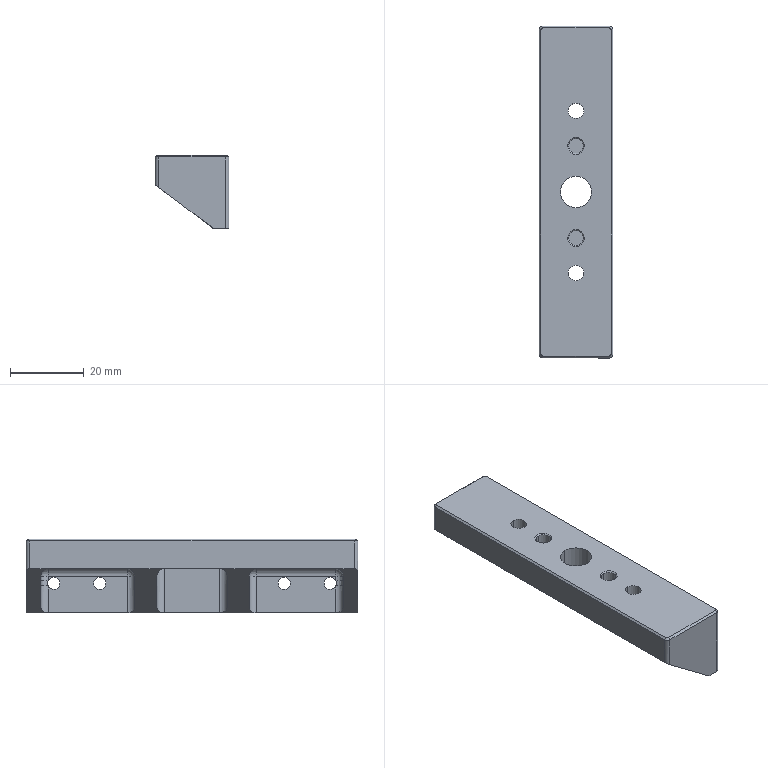NC program | NX | posted with a generic post | part box 20 x 90 x 20 mm
Lines 1 to 774 of 15930:
N10 G17 G21 G94 G90
(FLOOR_WALL_COPY , TOOL : D80)
N12 T19 M6
N14 G54
N16 G17 G0 G90 X-88. Y0. B0. C0. S6500 M3
N18 G43 Z30. H19
N20 Z7.
N22 G94 G1 Z4. F1500.
N24 X-85.
N26 X85.
N28 X88.
N30 Z7.
N32 G0 Z30.
N34 X-88.
N36 Z6.
N38 G1 Z3.
N40 X-85.
N42 X85.
N44 X88.
N46 Z6.
N48 G0 Z30.
N50 X-88.
N52 Z5.
N54 G1 Z2.
N56 X-85.
N58 X85.
N60 X88.
N62 Z5.
N64 G0 Z30.
N66 X-88.
N68 Z4.
N70 G1 Z1.
N72 X-85.
N74 X85.
N76 X88.
N78 Z4.
N80 G0 Z30.
N82 X-88.
N84 Z3.
N86 G1 Z0.
N88 X-85.
N90 X85.
N92 X88.
N94 Z3.
N96 G0 Z30.
N98 M5
(CAVITY_MILL , TOOL : D10)
N100 T15 M6
N102 G54
N104 G17 G0 G90 X4.33 Y-16.996 B0. C0. S9500 M3
N106 G43 Z30. H15
N108 Z0.508
N110 G94 G1 Z-0.992 F1000.
N112 X0.866 Y-10.996
N114 G3 X0. Y-10.496 R1.
N116 G1 Y-5.996
N118 X40.997 F3500.
N120 Y-4.989
N122 G2 X35.946 Y-3.6 R9.462
N124 G1 X20.574
N126 G2 X15.58 Y-4.989 R9.612
N128 G1 X9.359
N130 G2 X4.437 Y-3.6 R10.03
N132 G1 X-4.432
N134 G2 X-9.412 Y-4.989 R9.663
N136 G1 X-15.662
N138 G2 X-20.59 Y-3.6 R10.353
N140 G1 X-35.931
N142 G2 X-40.895 Y-4.989 R9.801
N144 G1 X-40.997
N146 Y-5.996
N148 X0.
N150 Y-10.496
N152 X45.004
N154 G3 X45.497 Y-10.003 R0.493
N156 G1 Y-1.867
N158 G3 X49.997 Y0.476 R6.533
N160 G1 Y3.622
N162 G2 X45. Y-0.489 R5.133
N164 G1 X40.881
N166 G2 X38.089 Y0.371 R4.962
N168 X37.347 Y0.9 R21.375
N170 G1 X19.1
N172 G2 X15.585 Y-0.489 R5.112
N174 G1 X9.409
N176 G2 X5.865 Y0.9 R5.53
N178 G1 X-5.9
N180 G2 X-9.415 Y-0.489 R5.163
N182 G1 X-15.591
N184 G2 X-19.194 Y0.9 R5.853
N186 G1 X-37.384
N188 G2 X-40.997 Y-0.489 R5.301
N190 G1 X-45.
N192 G2 X-49.997 Y3.622 R5.133
N194 G1 Y0.476
N196 G3 X-45.497 Y-1.867 R6.533
N198 G1 Y-10.003
N200 G3 X-45.004 Y-10.496 R0.493
N202 G1 X0.
N204 G2 X0.866 Y-10.996 R1.
N206 G1 X4.33 Y-16.996
N208 Z0.508
N210 G0 X32.575 Z-0.483
N212 G1 Z-1.983 F1000.
N214 X29.111 Y-10.996
N216 G3 X28.245 Y-10.496 R1.
N218 G1 Y-5.996
N220 X38.636 F3500.
N222 G2 X34.338 Y-3.6 R9.795
N224 G1 X22.164
N226 G2 X17.854 Y-5.996 R9.845
N228 G1 X28.245
N230 Y-10.496
N232 X45.004
N234 G3 X45.497 Y-10.003 R0.494
N236 G1 Y-3.187
N238 G3 X49.997 Y-0.827 R6.564
N240 G1 Y2.328
N242 G2 X45. Y-1.811 R5.164
N244 G1 X41.
N246 G2 X36.481 Y0.9 R5.295
N248 G1 X20.03
N250 G2 X15.5 Y-1.811 R5.345
N252 G1 X9.5
N254 G2 X8.216 Y-1.644 R5.087
N256 G1 X7.072 Y-5.996
N258 G2 X2.828 Y-3.6 R9.587
N260 G1 X-2.829
N262 G2 X-7.069 Y-5.996 R9.575
N264 G1 X7.072
N266 X8.216 Y-1.644
N268 G2 X5.011 Y0.9 R5.087
N270 G1 X-5.014
N272 G2 X-9.5 Y-1.811 R5.075
N274 G1 X-15.5
N276 G2 X-16.78 Y-1.644 R5.113
N278 G1 X-17.923 Y-5.996
N280 G2 X-22.174 Y-3.6 R9.613
N282 G1 X-34.338
N284 G2 X-38.636 Y-5.996 R9.795
N286 G1 X-17.923
N288 X-16.78 Y-1.644
N290 G2 X-19.996 Y0.9 R5.113
N292 G1 X-36.481
N294 G2 X-41. Y-1.811 R5.295
N296 G1 X-45.033
N298 G2 X-49.997 Y2.331 R5.167
N300 G1 Y-0.825
N302 G3 X-45.497 Y-3.187 R6.567
N304 G1 Y-10.003
N306 G3 X-45.004 Y-10.496 R0.494
N308 G1 X28.245
N310 G2 X29.111 Y-10.996 R1.
N312 G1 X32.575 Y-16.996
N314 Z-0.483
N316 G0 X32.581 Z-1.475
N318 G1 Z-2.975 F1000.
N320 X29.117 Y-10.996
N322 G3 X28.251 Y-10.496 R1.
N324 G1 Y-5.996
N326 X35.657 F3500.
N328 G2 X33.194 Y-3.6 R9.616
N330 G1 X23.307
N332 G2 X20.845 Y-5.996 R9.612
N334 G1 X28.251
N336 Y-10.496
N338 X45.004
N340 G3 X45.497 Y-10.002 R0.494
N342 G1 Y-4.512
N344 G3 X49.997 Y-2.169 R6.533
N346 G1 Y0.979
N348 G2 X45. Y-3.133 R5.133
N350 G1 X41.
N352 G2 X36.023 Y0.9 R5.116
N354 G1 X20.476
N356 G2 X15.5 Y-3.133 R5.112
N358 G1 X9.5
N360 G2 X6.666 Y-2.263 R5.105
N362 G1 X4.153 Y-5.996
N364 G2 X1.693 Y-3.6 R9.605
N366 G1 X-1.693
N368 G2 X-4.153 Y-5.996 R9.605
N370 G1 X4.153
N372 X6.666 Y-2.263
N374 G2 X4.525 Y0.9 R5.105
N376 G1 X-4.525
N378 G2 X-9.5 Y-3.133 R5.105
N380 G1 X-15.5
N382 G2 X-18.333 Y-2.263 R5.113
N384 G1 X-20.845 Y-5.996
N386 G2 X-23.307 Y-3.6 R9.613
N388 G1 X-33.194
N390 G2 X-35.656 Y-5.996 R9.615
N392 G1 X-20.845
N394 X-18.333 Y-2.263
N396 G2 X-20.477 Y0.9 R5.113
N398 G1 X-36.024
N400 G2 X-41. Y-3.133 R5.115
N402 G1 X-45.019
N404 G2 X-49.997 Y0.981 R5.136
N406 G1 Y-2.167
N408 G3 X-45.497 Y-4.512 R6.536
N410 G1 Y-10.002
N412 G3 X-45.004 Y-10.496 R0.494
N414 G1 X28.251
N416 G2 X29.117 Y-10.996 R1.
N418 G1 X32.581 Y-16.996
N420 Z-1.475
N422 G0 X32.58 Y-16.997 Z-2.467
N424 G1 Z-3.967 F1000.
N426 X29.116 Y-10.997
N428 G3 X28.25 Y-10.497 R1.
N430 G1 Y-5.997
N432 X34.087 F3500.
N434 G2 X32.402 Y-3.6 R9.633
N436 G1 X24.098
N438 G2 X22.413 Y-5.997 R9.633
N440 G1 X28.25
N442 Y-10.497
N444 X45.003
N446 G3 X45.498 Y-10.002 R0.494
N448 G1 Y-5.834
N450 G3 X49.998 Y-3.491 R6.533
N452 G1 Y-0.343
N454 G2 X45. Y-4.456 R5.133
N456 G1 X41.
N458 G2 X35.9 Y0.711 R5.133
N460 G1 Y0.9
N462 X20.6
N464 Y0.711
N466 G2 X15.5 Y-4.456 R5.133
N468 G1 X9.5
N470 G2 X5.832 Y-2.879 R5.133
N472 G1 X2.587 Y-5.997
N474 G2 X0.902 Y-3.6 R9.633
N476 G1 X-0.902
N478 G2 X-2.587 Y-5.997 R9.633
N480 G1 X2.587
N482 X5.832 Y-2.879
N484 G2 X4.517 Y-0.413 R5.133
N486 X4.4 Y0.756 R5.134
N488 G1 X4.401 Y0.9
N490 X-4.4
N492 Y0.711
N494 G2 X-9.5 Y-4.456 R5.133
N496 G1 X-15.5
N498 G2 X-19.168 Y-2.879 R5.133
N500 G1 X-22.413 Y-5.997
N502 G2 X-24.098 Y-3.6 R9.633
N504 G1 X-32.402
N506 G2 X-34.087 Y-5.997 R9.633
N508 G1 X-22.413
N510 X-19.168 Y-2.879
N512 G2 X-20.6 Y0.711 R5.133
N514 G1 Y0.9
N516 X-35.9
N518 Y0.711
N520 G2 X-41. Y-4.456 R5.133
N522 G1 X-45.
N524 G2 X-49.998 Y-0.343 R5.133
N526 G1 Y-3.491
N528 G3 X-45.498 Y-5.834 R6.533
N530 G1 Y-10.002
N532 G3 X-45.003 Y-10.497 R0.494
N534 G1 X28.25
N536 G2 X29.116 Y-10.997 R1.
N538 G1 X32.58 Y-16.997
N540 Z-2.467
N542 G0 X32.581 Z-3.458
N544 G1 Z-4.958 F1000.
N546 X29.117 Y-10.997
N548 G3 X28.251 Y-10.497 R1.
N550 G1 Y-5.997
N552 X33.027 F3500.
N554 G2 X31.867 Y-3.6 R9.641
N556 G1 X24.635
N558 G2 X23.475 Y-5.997 R9.636
N560 G1 X28.251
N562 Y-10.497
N564 X45.003
N566 G3 X45.498 Y-10.002 R0.494
N568 G1 Y-7.154
N570 G3 X49.998 Y-4.793 R6.565
N572 G1 Y-1.636
N574 G2 X45. Y-5.778 R5.165
N576 G1 X41.
N578 G2 X35.9 Y-0.611 R5.141
N580 G1 Y0.9
N582 X20.6
N584 Y-0.611
N586 G2 X15.5 Y-5.778 R5.136
N588 G1 X9.5
N590 G2 X5.279 Y-3.488 R5.175
N592 G1 X1.543 Y-5.997
N594 G2 X0.376 Y-3.6 R9.675
N596 G1 X-0.376
N598 G2 X-1.543 Y-5.997 R9.675
N600 G1 X1.543
N602 X5.279 Y-3.488
N604 G2 X4.4 Y-0.611 R5.175
N606 G1 Y0.9
N608 X-4.4
N610 Y-0.611
N612 G2 X-9.5 Y-5.778 R5.175
N614 G1 X-15.5
N616 G2 X-19.734 Y-3.496 R5.136
N618 G1 X-23.475 Y-5.997
N620 G2 X-24.635 Y-3.6 R9.636
N622 G1 X-31.867
N624 G2 X-33.027 Y-5.997 R9.641
N626 G1 X-23.475
N628 X-19.734 Y-3.496
N630 G2 X-20.6 Y-0.611 R5.136
N632 G1 Y0.9
N634 X-35.9
N636 Y-0.611
N638 G2 X-41. Y-5.778 R5.141
N640 G1 X-45.
N642 G2 X-49.998 Y-1.634 R5.167
N644 G1 Y-4.791
N646 G3 X-45.498 Y-7.154 R6.567
N648 G1 Y-10.002
N650 G3 X-45.003 Y-10.497 R0.494
N652 G1 X28.251
N654 G2 X29.117 Y-10.997 R1.
N656 G1 X32.581 Y-16.997
N658 Z-3.458
N660 G0 X32.582 Z-4.45
N662 G1 Z-5.95 F1000.
N664 X29.118 Y-10.997
N666 G3 X28.252 Y-10.497 R1.
N668 G1 Y-5.997
N670 X32.287 F3500.
N672 G2 X31.541 Y-3.6 R9.644
N674 G1 X24.961
N676 G2 X24.217 Y-5.997 R9.633
N678 G1 X28.252
N680 Y-10.497
N682 X45.003
N684 G3 X45.498 Y-10.002 R0.495
N686 G1 Y-8.478
N688 G3 X49.998 Y-6.129 R6.543
N690 G1 Y-2.977
N692 G2 X45. Y-7.1 R5.143
N694 G1 X41.
N696 G2 X35.9 Y-1.933 R5.144
N698 G1 Y0.9
N700 X20.6
N702 Y-1.933
N704 G2 X15.5 Y-7.1 R5.133
N706 G1 X9.5
N708 G2 X4.879 Y-4.105 R5.17
N710 G1 X0.797 Y-5.997
N712 G2 X0.045 Y-3.6 R9.67
N714 G1 X-0.045
N716 G2 X-0.797 Y-5.997 R9.67
N718 G1 X0.797
N720 X4.879 Y-4.105
N722 G2 X4.4 Y-1.933 R5.17
N724 G1 Y0.9
N726 X-4.4
N728 Y-1.933
N730 G2 X-9.5 Y-7.1 R5.17
N732 G1 X-15.533
N734 G2 X-20.129 Y-4.114 R5.133
N736 G1 X-24.217 Y-5.997
N738 G2 X-24.961 Y-3.6 R9.633
N740 G1 X-31.541
N742 G2 X-32.287 Y-5.997 R9.644
N744 G1 X-24.217
N746 X-20.129 Y-4.114
N748 G2 X-20.6 Y-1.933 R5.133
N750 G1 Y0.9
N752 X-35.9
N754 Y-1.933
N756 G2 X-41. Y-7.1 R5.144
N758 G1 X-45.
N760 G2 X-49.998 Y-2.975 R5.146
N762 G1 Y-6.127
N764 G3 X-45.498 Y-8.478 R6.546
N766 G1 Y-10.002
N768 G3 X-45.003 Y-10.497 R0.495
N770 G1 X28.252
N772 G2 X29.118 Y-10.997 R1.
N774 G1 X32.582 Y-16.997
N776 Z-4.45
N778 G0 X32.58 Z-5.442
N780 G1 Z-6.942 F1000.
N782 X29.116 Y-10.997
N784 G3 X28.25 Y-10.497 R1.
N786 G1 Y-5.997
N788 X31.788 F3500.
N790 G2 X31.405 Y-3.6 R9.633
N792 G1 X25.095
N794 G2 X24.712 Y-5.997 R9.633
N796 G1 X28.25
N798 Y-10.497
N800 X45.003
N802 G3 X45.498 Y-10.002 R0.495
N804 G1 Y-9.801
N806 G3 X49.998 Y-7.457 R6.533
N808 G1 Y-4.307
N810 G2 X45. Y-8.422 R5.133
N812 G1 X41.
N814 G2 X35.9 Y-3.256 R5.133
N816 G1 Y0.9
N818 X20.6
N820 Y-3.256
N822 G2 X15.5 Y-8.422 R5.133
N824 G1 X9.5
N826 G2 X4.607 Y-4.732 R5.133
N828 G1 X0.288 Y-5.997
N830 G2 X0. Y-4.674 R9.633
N832 X-0.288 Y-5.997 R9.633
N834 G1 X0.288
N836 X4.607 Y-4.732
N838 G2 X4.4 Y-3.256 R5.133
N840 G1 Y0.9
N842 X-4.4
N844 Y-3.256
N846 G2 X-9.5 Y-8.422 R5.133
N848 G1 X-15.5
N850 G2 X-20.393 Y-4.732 R5.133
N852 G1 X-24.712 Y-5.997
N854 G2 X-25.095 Y-3.6 R9.633
N856 G1 X-31.405
N858 G2 X-31.788 Y-5.997 R9.633
N860 G1 X-24.712
N862 X-20.393 Y-4.732
N864 G2 X-20.6 Y-3.256 R5.133
N866 G1 Y0.9
N868 X-35.9
N870 Y-3.256
N872 G2 X-41. Y-8.422 R5.133
N874 G1 X-45.
N876 G2 X-49.998 Y-4.307 R5.133
N878 G1 Y-7.457
N880 G3 X-45.498 Y-9.801 R6.533
N882 G1 Y-10.002
N884 G3 X-45.003 Y-10.497 R0.495
N886 G1 X28.25
N888 G2 X29.116 Y-10.997 R1.
N890 G1 X32.58 Y-16.997
N892 Z-5.442
N894 G0 Z-6.433
N896 G1 Z-7.933 F1000.
N898 X29.116 Y-10.997
N900 G3 X28.25 Y-10.497 R1.
N902 G1 Y-5.997
N904 X31.5 F3500.
N906 G2 X31.4 Y-4.674 R9.633
N908 G1 Y-3.6
N910 X25.1
N912 Y-4.565
N914 G2 X25. Y-5.997 R9.633
N916 G1 X28.25
N918 Y-10.497
N920 X38.198
N922 G3 X41. Y-11.144 R6.533
N924 G1 X45.012
N926 G3 X49.998 Y-8.772 R6.544
N928 G1 Y-5.619
N930 G2 X45. Y-9.744 R5.144
N932 G1 X41.
N934 G2 X35.9 Y-4.578 R5.133
N936 G1 Y0.9
N938 X20.6
N940 Y-4.644
N942 G2 X15.5 Y-9.744 R5.133
N944 G1 X9.5
N946 G2 X4.454 Y-5.346 R5.143
N948 G1 X0.001 Y-5.997
N950 X4.454 Y-5.346
N952 X4.453 Y-5.341
N954 G2 X4.4 Y-4.578 R5.143
N956 G1 Y0.9
N958 X-4.4
N960 Y-4.578
N962 G2 X-9.5 Y-9.744 R5.143
N964 G1 X-15.5
N966 G2 X-20.547 Y-5.35 R5.133
N968 G1 X-25. Y-5.997
N970 G2 X-25.1 Y-4.674 R9.633
N972 G1 Y-3.6
N974 X-31.4
N976 Y-4.565
N978 G2 X-31.5 Y-5.997 R9.633
N980 G1 X-25.
N982 X-20.547 Y-5.35
N984 G2 X-20.6 Y-4.578 R5.133
N986 G1 Y0.9
N988 X-35.9
N990 Y-4.644
N992 G2 X-41. Y-9.744 R5.133
N994 G1 X-45.
N996 G2 X-49.998 Y-5.617 R5.146
N998 G1 Y-8.771
N1000 G3 X-45. Y-11.144 R6.546
N1002 G1 X-40.991
N1004 G3 X-38.198 Y-10.497 R6.533
N1006 G1 X-18.302
N1008 G3 X-15.5 Y-11.144 R6.533
N1010 G1 X-9.488
N1012 G3 X-6.705 Y-10.497 R6.543
N1014 G1 X6.705
N1016 G3 X9.5 Y-11.144 R6.543
N1018 G1 X15.509
N1020 G3 X18.302 Y-10.497 R6.533
N1022 G1 X28.25
N1024 G2 X29.116 Y-10.997 R1.
N1026 G1 X32.58 Y-16.997
N1028 Z-6.433
N1030 G0 Z-7.425
N1032 G1 Z-8.925 F1000.
N1034 X29.116 Y-10.997
N1036 G3 X28.25 Y-10.497 R1.
N1038 G1 Y-5.997
N1040 X31.4 F3500.
N1042 Y-5.893
N1044 Y-3.6
N1046 X25.1
N1048 Y-5.888
N1050 Y-5.997
N1052 X28.25
N1054 Y-10.497
N1056 X36.366
N1058 G3 X41. Y-12.467 R6.547
N1060 G1 X45.016
N1062 G3 X49.872 Y-10.232 R6.56
N1064 X49.998 Y-9.14 R6.
N1066 G1 Y-6.926
N1068 G2 X45. Y-11.067 R5.16
N1070 G1 X41.
N1072 G2 X35.9 Y-5.9 R5.147
N1074 G1 Y0.9
N1076 X20.6
N1078 Y-0.5
N1080 Y-5.967
N1082 G2 X15.5 Y-11.067 R5.135
N1084 G1 X9.5
N1086 G2 X4.4 Y-5.9 R5.182
N1088 G1 Y0.9
N1090 X-4.4
N1092 Y-5.9
N1094 G2 X-9.5 Y-11.067 R5.182
N1096 G1 X-15.5
N1098 G2 X-20.6 Y-5.967 R5.135
N1100 G1 X-25.1 Y-5.997
N1102 Y-5.888
N1104 Y-3.6
N1106 X-31.4
N1108 Y-5.893
N1110 Y-5.997
N1112 X-25.1
N1114 X-20.6 Y-5.967
N1116 Y-0.5
N1118 Y0.9
N1120 X-35.9
N1122 Y-0.5
N1124 Y-5.961
N1126 G2 X-41. Y-11.067 R5.147
N1128 G1 X-45.
N1130 G2 X-49.998 Y-6.923 R5.163
N1132 G1 Y-9.14
N1134 G3 X-49.873 Y-10.23 R6.
N1136 X-45. Y-12.467 R6.563
N1138 G1 X-40.987
N1140 G3 X-36.366 Y-10.497 R6.547
N1142 G1 X-20.141
N1144 G3 X-15.5 Y-12.467 R6.535
N1146 G1 X-9.478 Y-12.466
N1148 G3 X-4.886 Y-10.497 R6.582
N1150 G1 X4.886
N1152 G3 X9.5 Y-12.467 R6.582
N1154 G1 X15.51
N1156 G3 X20.141 Y-10.497 R6.535
N1158 G1 X28.25
N1160 G2 X29.116 Y-10.997 R1.
N1162 G1 X32.58 Y-16.997
N1164 Z-7.425
N1166 G0 Y-16.998 Z-8.417
N1168 G1 Z-9.917 F1000.
N1170 X29.116 Y-10.998
N1172 G3 X28.25 Y-10.498 R1.
N1174 G1 Y-5.998
N1176 X31.4 F3500.
N1178 Y-3.6
N1180 X25.1
N1182 Y-5.998
N1184 X28.25
N1186 Y-10.498
N1188 X35.361
N1190 G3 X41. Y-13.789 R6.533
N1192 G1 X45.009
N1194 G3 X48.885 Y-12.483 R6.533
N1196 X49.999 Y-9.133 R6.
N1198 G1 Y-8.272
N1200 G2 X45. Y-12.389 R5.133
N1202 G1 X41.
N1204 G2 X35.9 Y-7.222 R5.133
N1206 G1 Y0.9
N1208 X20.6
N1210 Y-7.222
N1212 G2 X15.5 Y-12.389 R5.133
N1214 G1 X9.5
N1216 G2 X4.4 Y-7.222 R5.152
N1218 G1 Y0.9
N1220 X-4.4
N1222 Y-7.222
N1224 G2 X-9.5 Y-12.389 R5.133
N1226 G1 X-15.5
N1228 G2 X-20.6 Y-7.222 R5.133
N1230 G1 Y-5.998
N1232 X-25.1
N1234 Y-3.6
N1236 X-31.4
N1238 Y-5.998
N1240 X-25.1
N1242 X-20.6
N1244 Y0.9
N1246 X-35.9
N1248 Y-7.222
N1250 G2 X-41. Y-12.389 R5.133
N1252 G1 X-45.042 Y-12.388
N1254 G2 X-49.999 Y-8.272 R5.133
N1256 G1 Y-9.133
N1258 G3 X-48.885 Y-12.483 R6.
N1260 X-45. Y-13.789 R6.533
N1262 G1 X-40.991
N1264 G3 X-35.361 Y-10.498 R6.533
N1266 G1 X-21.139
N1268 G3 X-15.5 Y-13.789 R6.533
N1270 G1 X-9.491
N1272 G3 X-3.861 Y-10.498 R6.533
N1274 G1 X3.869
N1276 G3 X9.5 Y-13.789 R6.552
N1278 G1 X15.509
N1280 G3 X21.139 Y-10.498 R6.533
N1282 G1 X28.25
N1284 G2 X29.116 Y-10.998 R1.
N1286 G1 X32.58 Y-16.998
N1288 Z-8.417
N1290 G0 Z-9.408
N1292 G1 Z-10.908 F1000.
N1294 X29.116 Y-10.998
N1296 G3 X28.25 Y-10.498 R1.
N1298 G1 Y-5.998
N1300 X31.169 F3500.
N1302 Y-3.831
N1304 X25.331
N1306 Y-5.998
N1308 X28.25
N1310 Y-10.498
N1312 X34.545
N1314 G3 X39.548 Y-14.998 R6.486
N1316 G1 X44.165
N1318 G3 X49.942 Y-9.834 R6.
N1320 G2 X45. Y-13.711 R5.144
N1322 G1 X40.735
N1324 G2 X35.669 Y-8.605 R5.086
N1326 G1 Y0.669
N1328 X20.831
N1330 Y-8.606
N1332 G2 X15.761 Y-13.711 R5.087
N1334 G1 X9.222
N1336 G2 X4.169 Y-8.605 R5.086
N1338 G1 Y0.9
N1340 X-4.169
N1342 Y-8.606
N1344 G2 X-9.239 Y-13.711 R5.087
N1346 G1 X-15.779
N1348 G2 X-20.831 Y-8.659 R5.052
N1350 G1 Y-5.998
N1352 X-25.331
N1354 Y-3.831
N1356 X-31.169
N1358 Y-5.998
N1360 X-25.331
N1362 X-20.831
N1364 Y0.669
N1366 X-35.669
N1368 Y-8.606
N1370 G2 X-40.739 Y-13.711 R5.087
N1372 G1 X-45.
N1374 G2 X-49.944 Y-9.821 R5.15
N1376 G3 X-44.165 Y-14.998 R6.
N1378 G1 X-39.548
N1380 G3 X-34.545 Y-10.498 R6.487
N1382 G1 X-21.964
N1384 G3 X-16.983 Y-14.998 R6.452
N1386 G1 X-8.048
N1388 G3 X-3.045 Y-10.498 R6.487
N1390 G1 X3.045
N1392 G3 X8.048 Y-14.998 R6.486
N1394 G1 X16.952
N1396 G3 X21.955 Y-10.498 R6.487
N1398 G1 X28.25
N1400 G2 X29.116 Y-10.998 R1.
N1402 G1 X32.58 Y-16.998
N1404 Z-9.408
N1406 G0 X-23.92 Z-10.4
N1408 G1 Z-11.9 F1000.
N1410 X-27.384 Y-10.998
N1412 G3 X-28.25 Y-10.498 R1.
N1414 G1 Y-5.998
N1416 X-26.831 F3500.
N1418 Y-5.331
N1420 X-29.669
N1422 Y-5.998
N1424 X-28.25
N1426 Y-10.498
N1428 X-23.706
N1430 G3 X-21.295 Y-14.998 R6.498
N1432 G1 X-17.745
N1434 G2 X-22.331 Y-9.982 R5.098
N1436 G1 Y-0.831
N1438 X-34.169
N1440 Y-9.989
N1442 G2 X-38.753 Y-14.998 R5.096
N1444 G1 X-35.204
N1446 G3 X-32.793 Y-10.498 R6.496
N1448 G1 X-28.25
N1450 G2 X-27.384 Y-10.998 R1.
N1452 G1 X-23.92 Y-16.998
N1454 Z-10.4
N1456 G0 Z30.
N1458 X8.715 Y-17.023
N1460 Z-10.4
N1462 G1 Z-11.9 F1000.
N1464 X8.066 Y-15.582
N1466 G3 X7.255 Y-14.998 R1.
N1468 G2 X2.669 Y-9.982 R5.098 F3500.
N1470 G1 Y0.9
N1472 X-2.669
N1474 Y-9.989
N1476 G2 X-7.253 Y-14.998 R5.096
N1478 G3 X-8.064 Y-15.582 R1.
N1480 G1 X-8.713 Y-17.023
N1482 Z-10.4
N1484 G0 Z30.
N1486 X32.58 Y-16.998
N1488 Z-10.4
N1490 G1 Z-11.9 F1000.
N1492 X29.116 Y-10.998
N1494 G3 X28.25 Y-10.498 R1.
N1496 G1 Y-5.998
N1498 X29.669 F3500.
N1500 Y-5.331
N1502 X26.831
N1504 Y-5.998
N1506 X28.25
N1508 Y-10.498
N1510 X32.794
N1512 G3 X35.205 Y-14.998 R6.498
N1514 G1 X38.755
N1516 G2 X34.169 Y-9.982 R5.098
N1518 G1 Y-0.831
N1520 X22.331
N1522 Y-9.989
N1524 G2 X17.747 Y-14.998 R5.096
N1526 G1 X21.296
N1528 G3 X23.707 Y-10.498 R6.496
N1530 G1 X28.25
N1532 G2 X29.116 Y-10.998 R1.
N1534 G1 X32.58 Y-16.998
N1536 Z-10.4
N1538 G0 Z30.
N1540 M5